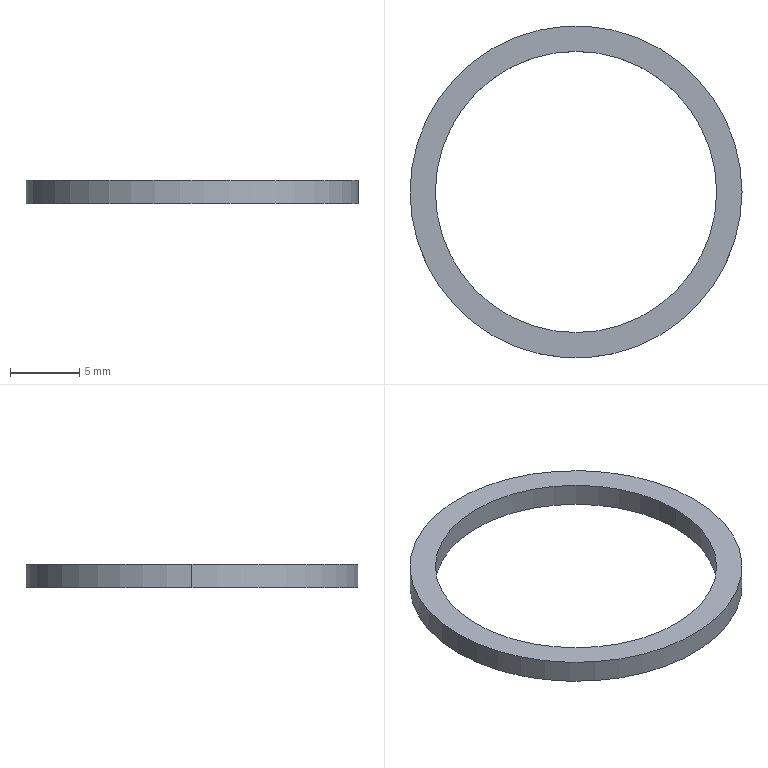Part | NX | features BREP 1 | 1 solid | 6 faces | box 23.91 x 23.91 x 1.67 mm | volume 211.991 mm3 | cylinder 4 | plane 2 | commonest cylinder face diameters 20.25 x2 23.91 x2
STEP:
#1=CARTESIAN_POINT('',(-284.419,27.798,0.));
#2=VERTEX_POINT('',#1);
#3=CARTESIAN_POINT('',(-264.169,27.798,0.));
#4=VERTEX_POINT('',#3);
#5=CARTESIAN_POINT('',(-274.294,27.798,0.));
#6=DIRECTION('',(0.,0.,1.));
#7=DIRECTION('',(1.,0.,0.));
#8=AXIS2_PLACEMENT_3D('',#5,#6,#7);
#9=CIRCLE('',#8,10.125);
#10=EDGE_CURVE('',#2,#4,#9,.T.);
#11=ORIENTED_EDGE('',*,*,#10,.F.);
#12=CARTESIAN_POINT('',(-284.419,27.798,1.67));
#13=VERTEX_POINT('',#12);
#14=CARTESIAN_POINT('',(-284.419,27.798,-8.5));
#15=DIRECTION('',(0.,0.,1.));
#16=VECTOR('',#15,1000.);
#17=LINE('',#14,#16);
#18=EDGE_CURVE('',#2,#13,#17,.T.);
#19=ORIENTED_EDGE('',*,*,#18,.T.);
#20=CARTESIAN_POINT('',(-264.169,27.798,1.67));
#21=VERTEX_POINT('',#20);
#22=CARTESIAN_POINT('',(-274.294,27.798,1.67));
#23=DIRECTION('',(0.,0.,1.));
#24=DIRECTION('',(1.,0.,0.));
#25=AXIS2_PLACEMENT_3D('',#22,#23,#24);
#26=CIRCLE('',#25,10.125);
#27=EDGE_CURVE('',#13,#21,#26,.T.);
#28=ORIENTED_EDGE('',*,*,#27,.T.);
#29=CARTESIAN_POINT('',(-264.169,27.798,-8.5));
#30=DIRECTION('',(0.,0.,1.));
#31=VECTOR('',#30,1000.);
#32=LINE('',#29,#31);
#33=EDGE_CURVE('',#4,#21,#32,.T.);
#34=ORIENTED_EDGE('',*,*,#33,.F.);
#35=EDGE_LOOP('',(#11,#19,#28,#34));
#36=FACE_BOUND('',#35,.T.);
#37=CARTESIAN_POINT('',(-274.294,27.798,-8.5));
#38=DIRECTION('',(0.,0.,1.));
#39=DIRECTION('',(-1.,0.,0.));
#40=AXIS2_PLACEMENT_3D('',#37,#38,#39);
#41=CYLINDRICAL_SURFACE('',#40,10.125);
#42=ADVANCED_FACE('',(#36),#41,.F.);
#43=CARTESIAN_POINT('',(-262.339,27.798,1.67));
#44=VERTEX_POINT('',#43);
#45=CARTESIAN_POINT('',(-286.249,27.798,1.67));
#46=VERTEX_POINT('',#45);
#47=CARTESIAN_POINT('',(-274.294,27.798,1.67));
#48=DIRECTION('',(0.,0.,1.));
#49=DIRECTION('',(1.,0.,0.));
#50=AXIS2_PLACEMENT_3D('',#47,#48,#49);
#51=CIRCLE('',#50,11.955);
#52=EDGE_CURVE('',#44,#46,#51,.T.);
#53=ORIENTED_EDGE('',*,*,#52,.F.);
#54=CARTESIAN_POINT('',(-262.339,27.798,0.));
#55=VERTEX_POINT('',#54);
#56=CARTESIAN_POINT('',(-262.339,27.798,1.5));
#57=DIRECTION('',(0.,0.,-1.));
#58=VECTOR('',#57,1000.);
#59=LINE('',#56,#58);
#60=EDGE_CURVE('',#55,#44,#59,.F.);
#61=ORIENTED_EDGE('',*,*,#60,.F.);
#62=CARTESIAN_POINT('',(-286.249,27.798,0.));
#63=VERTEX_POINT('',#62);
#64=CARTESIAN_POINT('',(-274.294,27.798,0.));
#65=DIRECTION('',(0.,0.,1.));
#66=DIRECTION('',(1.,0.,0.));
#67=AXIS2_PLACEMENT_3D('',#64,#65,#66);
#68=CIRCLE('',#67,11.955);
#69=EDGE_CURVE('',#55,#63,#68,.T.);
#70=ORIENTED_EDGE('',*,*,#69,.T.);
#71=CARTESIAN_POINT('',(-286.249,27.798,1.5));
#72=DIRECTION('',(0.,0.,-1.));
#73=VECTOR('',#72,1000.);
#74=LINE('',#71,#73);
#75=EDGE_CURVE('',#63,#46,#74,.F.);
#76=ORIENTED_EDGE('',*,*,#75,.T.);
#77=EDGE_LOOP('',(#53,#61,#70,#76));
#78=FACE_BOUND('',#77,.T.);
#79=CARTESIAN_POINT('',(-274.294,27.798,1.5));
#80=DIRECTION('',(0.,0.,-1.));
#81=DIRECTION('',(1.,0.,0.));
#82=AXIS2_PLACEMENT_3D('',#79,#80,#81);
#83=CYLINDRICAL_SURFACE('',#82,11.955);
#84=ADVANCED_FACE('',(#78),#83,.T.);
#85=CARTESIAN_POINT('',(-274.294,27.798,1.67));
#86=DIRECTION('',(0.,0.,1.));
#87=DIRECTION('',(1.,0.,0.));
#88=AXIS2_PLACEMENT_3D('',#85,#86,#87);
#89=CIRCLE('',#88,11.955);
#90=EDGE_CURVE('',#46,#44,#89,.T.);
#91=ORIENTED_EDGE('',*,*,#90,.T.);
#92=ORIENTED_EDGE('',*,*,#52,.T.);
#93=EDGE_LOOP('',(#91,#92));
#94=FACE_BOUND('',#93,.T.);
#95=CARTESIAN_POINT('',(-274.294,27.798,1.67));
#96=DIRECTION('',(0.,0.,1.));
#97=DIRECTION('',(1.,0.,0.));
#98=AXIS2_PLACEMENT_3D('',#95,#96,#97);
#99=CIRCLE('',#98,10.125);
#100=EDGE_CURVE('',#21,#13,#99,.T.);
#101=ORIENTED_EDGE('',*,*,#100,.F.);
#102=ORIENTED_EDGE('',*,*,#27,.F.);
#103=EDGE_LOOP('',(#101,#102));
#104=FACE_BOUND('',#103,.T.);
#105=CARTESIAN_POINT('',(-274.294,27.798,1.67));
#106=DIRECTION('',(0.,0.,1.));
#107=DIRECTION('',(-1.,0.,0.));
#108=AXIS2_PLACEMENT_3D('',#105,#106,#107);
#109=PLANE('',#108);
#110=ADVANCED_FACE('',(#94,#104),#109,.T.);
#111=CARTESIAN_POINT('',(-274.294,27.798,0.));
#112=DIRECTION('',(0.,0.,1.));
#113=DIRECTION('',(1.,0.,0.));
#114=AXIS2_PLACEMENT_3D('',#111,#112,#113);
#115=CIRCLE('',#114,11.955);
#116=EDGE_CURVE('',#63,#55,#115,.T.);
#117=ORIENTED_EDGE('',*,*,#116,.F.);
#118=ORIENTED_EDGE('',*,*,#69,.F.);
#119=EDGE_LOOP('',(#117,#118));
#120=FACE_BOUND('',#119,.T.);
#121=CARTESIAN_POINT('',(-274.294,27.798,0.));
#122=DIRECTION('',(0.,0.,1.));
#123=DIRECTION('',(1.,0.,0.));
#124=AXIS2_PLACEMENT_3D('',#121,#122,#123);
#125=CIRCLE('',#124,10.125);
#126=EDGE_CURVE('',#4,#2,#125,.T.);
#127=ORIENTED_EDGE('',*,*,#126,.T.);
#128=ORIENTED_EDGE('',*,*,#10,.T.);
#129=EDGE_LOOP('',(#127,#128));
#130=FACE_BOUND('',#129,.T.);
#131=CARTESIAN_POINT('',(-274.294,27.798,0.));
#132=DIRECTION('',(0.,0.,1.));
#133=DIRECTION('',(-1.,0.,0.));
#134=AXIS2_PLACEMENT_3D('',#131,#132,#133);
#135=PLANE('',#134);
#136=ADVANCED_FACE('',(#120,#130),#135,.F.);
#137=ORIENTED_EDGE('',*,*,#60,.T.);
#138=ORIENTED_EDGE('',*,*,#90,.F.);
#139=ORIENTED_EDGE('',*,*,#75,.F.);
#140=ORIENTED_EDGE('',*,*,#116,.T.);
#141=EDGE_LOOP('',(#137,#138,#139,#140));
#142=FACE_BOUND('',#141,.T.);
#143=CARTESIAN_POINT('',(-274.294,27.798,1.5));
#144=DIRECTION('',(0.,0.,-1.));
#145=DIRECTION('',(1.,0.,0.));
#146=AXIS2_PLACEMENT_3D('',#143,#144,#145);
#147=CYLINDRICAL_SURFACE('',#146,11.955);
#148=ADVANCED_FACE('',(#142),#147,.T.);
#149=ORIENTED_EDGE('',*,*,#18,.F.);
#150=ORIENTED_EDGE('',*,*,#126,.F.);
#151=ORIENTED_EDGE('',*,*,#33,.T.);
#152=ORIENTED_EDGE('',*,*,#100,.T.);
#153=EDGE_LOOP('',(#149,#150,#151,#152));
#154=FACE_BOUND('',#153,.T.);
#155=CARTESIAN_POINT('',(-274.294,27.798,-8.5));
#156=DIRECTION('',(0.,0.,1.));
#157=DIRECTION('',(-1.,0.,0.));
#158=AXIS2_PLACEMENT_3D('',#155,#156,#157);
#159=CYLINDRICAL_SURFACE('',#158,10.125);
#160=ADVANCED_FACE('',(#154),#159,.F.);
#161=CLOSED_SHELL('',(#42,#84,#110,#136,#148,#160));
#162=MANIFOLD_SOLID_BREP('',#161);
#163=(LENGTH_UNIT()NAMED_UNIT(*)SI_UNIT(.MILLI.,.METRE.));
#164=UNCERTAINTY_MEASURE_WITH_UNIT(LENGTH_MEASURE(0.00001),#163,'','');
#165=(NAMED_UNIT(*)PLANE_ANGLE_UNIT()SI_UNIT($,.RADIAN.));
#166=(NAMED_UNIT(*)SI_UNIT($,.STERADIAN.)SOLID_ANGLE_UNIT());
#167=(GEOMETRIC_REPRESENTATION_CONTEXT(3)GLOBAL_UNCERTAINTY_ASSIGNED_CONTEXT((#164))GLOBAL_UNIT_ASSIGNED_CONTEXT((#163,#165,#166))REPRESENTATION_CONTEXT('',''));
#168=ADVANCED_BREP_SHAPE_REPRESENTATION('',(#162),#167);